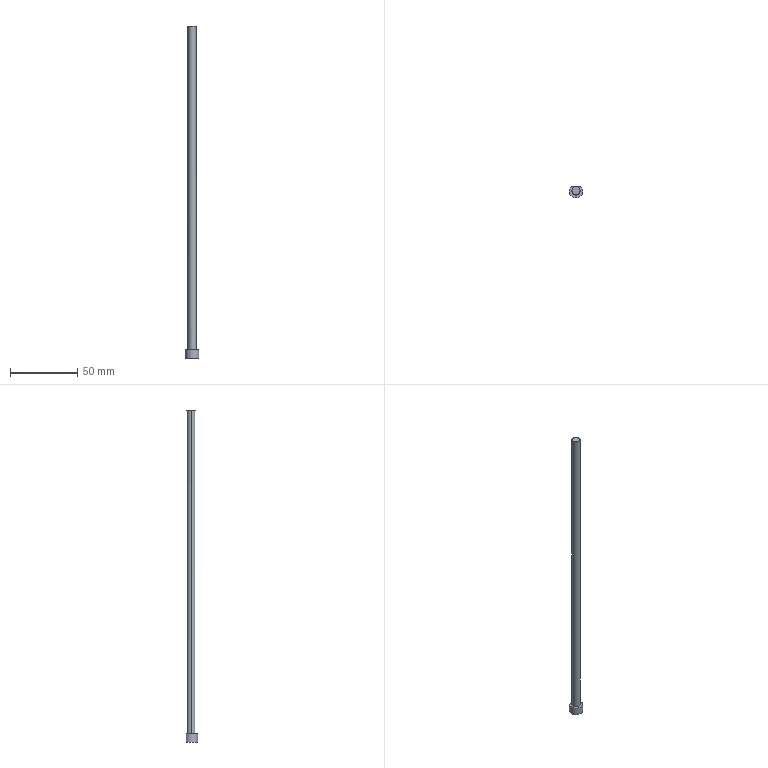Part | Creo | 1 solid | 7 faces | box 10 x 8.5 x 247.026 mm | volume 7242 mm3 | plane 4 | cylinder 3 | commonest cylinder face diameters 6 x2 10 x1
STEP:
#1=CARTESIAN_POINT('',(0.,0.,0.));
#2=DIRECTION('',(0.,0.,1.));
#3=DIRECTION('',(1.,0.,0.));
#4=AXIS2_PLACEMENT_3D('',#1,#2,#3);
#5=CARTESIAN_POINT('',(-69.606,-19.357,-332.441));
#6=VERTEX_POINT('',#5);
#7=CARTESIAN_POINT('',(-76.747,-19.357,-332.441));
#8=VERTEX_POINT('',#7);
#9=CARTESIAN_POINT('',(-69.606,-19.357,-332.441));
#10=DIRECTION('',(-1.,0.,0.));
#11=VECTOR('',#10,7.141);
#12=LINE('',#9,#11);
#13=EDGE_CURVE('',#6,#8,#12,.T.);
#14=ORIENTED_EDGE('',*,*,#13,.F.);
#15=CARTESIAN_POINT('',(-73.177,-22.857,-332.441));
#16=DIRECTION('',(0.,0.,-1.));
#17=DIRECTION('',(0.7141,0.7,0.));
#18=AXIS2_PLACEMENT_3D('',#15,#16,#17);
#19=CIRCLE('',#18,5.);
#20=EDGE_CURVE('',#6,#8,#19,.T.);
#21=ORIENTED_EDGE('',*,*,#20,.T.);
#22=EDGE_LOOP('',(#14,#21));
#23=FACE_OUTER_BOUND('',#22,.F.);
#24=CARTESIAN_POINT('',(-76.177,-22.857,-332.441));
#25=VERTEX_POINT('',#24);
#26=CARTESIAN_POINT('',(-70.177,-22.857,-332.441));
#27=VERTEX_POINT('',#26);
#28=CARTESIAN_POINT('',(-73.177,-22.857,-332.441));
#29=DIRECTION('',(0.,0.,-1.));
#30=DIRECTION('',(-1.,0.,0.));
#31=AXIS2_PLACEMENT_3D('',#28,#29,#30);
#32=CIRCLE('',#31,3.);
#33=EDGE_CURVE('',#25,#27,#32,.T.);
#34=ORIENTED_EDGE('',*,*,#33,.F.);
#35=CARTESIAN_POINT('',(-73.177,-22.857,-332.441));
#36=DIRECTION('',(0.,0.,-1.));
#37=DIRECTION('',(1.,0.,0.));
#38=AXIS2_PLACEMENT_3D('',#35,#36,#37);
#39=CIRCLE('',#38,3.);
#40=EDGE_CURVE('',#27,#25,#39,.T.);
#41=ORIENTED_EDGE('',*,*,#40,.F.);
#42=EDGE_LOOP('',(#34,#41));
#43=FACE_BOUND('',#42,.F.);
#44=CARTESIAN_POINT('',(-73.177,-22.857,-332.441));
#45=DIRECTION('',(0.,0.,-1.));
#46=DIRECTION('',(-1.,0.,0.));
#47=AXIS2_PLACEMENT_3D('',#44,#45,#46);
#48=PLANE('',#47);
#49=ADVANCED_FACE('',(#23,#43),#48,.F.);
#50=CARTESIAN_POINT('',(-70.177,-22.857,-91.423));
#51=VERTEX_POINT('',#50);
#52=CARTESIAN_POINT('',(-76.177,-22.856,-91.415));
#53=VERTEX_POINT('',#52);
#54=CARTESIAN_POINT('',(-70.177,-22.857,-91.423));
#55=CARTESIAN_POINT('',(-70.177,-22.528,-91.423));
#56=CARTESIAN_POINT('',(-70.279,-21.908,-91.423));
#57=CARTESIAN_POINT('',(-70.718,-21.051,-91.422));
#58=CARTESIAN_POINT('',(-71.395,-20.383,-91.421));
#59=CARTESIAN_POINT('',(-72.241,-19.955,-91.42));
#60=CARTESIAN_POINT('',(-73.175,-19.808,-91.419));
#61=CARTESIAN_POINT('',(-74.109,-19.954,-91.418));
#62=CARTESIAN_POINT('',(-74.956,-20.381,-91.417));
#63=CARTESIAN_POINT('',(-75.633,-21.048,-91.416));
#64=CARTESIAN_POINT('',(-76.073,-21.903,-91.415));
#65=CARTESIAN_POINT('',(-76.177,-22.527,-91.415));
#66=CARTESIAN_POINT('',(-76.177,-22.856,-91.415));
#67=B_SPLINE_CURVE_WITH_KNOTS('',3,(#54,#55,#56,#57,#58,#59,#60,#61,#62,#63,#64,#65,#66),.UNSPECIFIED.,.F.,.F.,(4,1,1,1,1,1,1,1,1,1,4),(0.,0.1,0.2,0.3,0.4,0.5,0.6,0.7,0.8,0.9,1.),.UNSPECIFIED.);
#68=EDGE_CURVE('',#51,#53,#67,.T.);
#69=ORIENTED_EDGE('',*,*,#68,.T.);
#70=CARTESIAN_POINT('',(-76.177,-22.857,-332.441));
#71=DIRECTION('',(0.000000003,0.000005265,1.));
#72=VECTOR('',#71,241.026);
#73=LINE('',#70,#72);
#74=EDGE_CURVE('',#25,#53,#73,.T.);
#75=ORIENTED_EDGE('',*,*,#74,.F.);
#76=ORIENTED_EDGE('',*,*,#33,.T.);
#77=CARTESIAN_POINT('',(-70.177,-22.857,-332.441));
#78=DIRECTION('',(0.,0.,1.));
#79=VECTOR('',#78,241.019);
#80=LINE('',#77,#79);
#81=EDGE_CURVE('',#27,#51,#80,.T.);
#82=ORIENTED_EDGE('',*,*,#81,.T.);
#83=EDGE_LOOP('',(#69,#75,#76,#82));
#84=FACE_OUTER_BOUND('',#83,.F.);
#85=CARTESIAN_POINT('',(-73.177,-22.857,-653.441));
#86=DIRECTION('',(0.,0.,1.));
#87=DIRECTION('',(1.,0.,0.));
#88=AXIS2_PLACEMENT_3D('',#85,#86,#87);
#89=CYLINDRICAL_SURFACE('',#88,3.);
#90=ADVANCED_FACE('',(#84),#89,.T.);
#91=CARTESIAN_POINT('',(-76.177,-22.856,-91.415));
#92=CARTESIAN_POINT('',(-76.177,-23.186,-91.415));
#93=CARTESIAN_POINT('',(-76.075,-23.804,-91.415));
#94=CARTESIAN_POINT('',(-75.636,-24.661,-91.416));
#95=CARTESIAN_POINT('',(-74.97,-25.322,-91.417));
#96=CARTESIAN_POINT('',(-74.131,-25.754,-91.418));
#97=CARTESIAN_POINT('',(-73.189,-25.907,-91.419));
#98=CARTESIAN_POINT('',(-72.247,-25.761,-91.42));
#99=CARTESIAN_POINT('',(-71.402,-25.336,-91.421));
#100=CARTESIAN_POINT('',(-70.725,-24.674,-91.422));
#101=CARTESIAN_POINT('',(-70.279,-23.807,-91.423));
#102=CARTESIAN_POINT('',(-70.177,-23.186,-91.423));
#103=CARTESIAN_POINT('',(-70.177,-22.857,-91.423));
#104=B_SPLINE_CURVE_WITH_KNOTS('',3,(#91,#92,#93,#94,#95,#96,#97,#98,#99,#100,#101,#102,#103),.UNSPECIFIED.,.F.,.F.,(4,1,1,1,1,1,1,1,1,1,4),(0.,0.1,0.2,0.3,0.4,0.5,0.6,0.7,0.8,0.9,1.),.UNSPECIFIED.);
#105=EDGE_CURVE('',#53,#51,#104,.T.);
#106=ORIENTED_EDGE('',*,*,#105,.F.);
#107=ORIENTED_EDGE('',*,*,#68,.F.);
#108=EDGE_LOOP('',(#106,#107));
#109=FACE_OUTER_BOUND('',#108,.F.);
#110=CARTESIAN_POINT('',(248.993,54.022,-91.842));
#111=DIRECTION('',(-0.001312,0.000001665,-1.));
#112=DIRECTION('',(-1.,0.,0.001312));
#113=AXIS2_PLACEMENT_3D('',#110,#111,#112);
#114=PLANE('',#113);
#115=ADVANCED_FACE('',(#109),#114,.F.);
#116=ORIENTED_EDGE('',*,*,#105,.T.);
#117=ORIENTED_EDGE('',*,*,#81,.F.);
#118=ORIENTED_EDGE('',*,*,#40,.T.);
#119=ORIENTED_EDGE('',*,*,#74,.T.);
#120=EDGE_LOOP('',(#116,#117,#118,#119));
#121=FACE_OUTER_BOUND('',#120,.F.);
#122=CARTESIAN_POINT('',(-73.177,-22.857,-653.441));
#123=DIRECTION('',(0.,0.,1.));
#124=DIRECTION('',(1.,0.,0.));
#125=AXIS2_PLACEMENT_3D('',#122,#123,#124);
#126=CYLINDRICAL_SURFACE('',#125,3.);
#127=ADVANCED_FACE('',(#121),#126,.T.);
#128=CARTESIAN_POINT('',(-76.747,-19.357,-338.441));
#129=VERTEX_POINT('',#128);
#130=CARTESIAN_POINT('',(-76.747,-19.357,-332.441));
#131=DIRECTION('',(0.,0.,-1.));
#132=VECTOR('',#131,6.);
#133=LINE('',#130,#132);
#134=EDGE_CURVE('',#8,#129,#133,.T.);
#135=ORIENTED_EDGE('',*,*,#134,.T.);
#136=CARTESIAN_POINT('',(-69.606,-19.357,-338.441));
#137=VERTEX_POINT('',#136);
#138=CARTESIAN_POINT('',(-69.606,-19.357,-338.441));
#139=DIRECTION('',(-1.,0.,0.));
#140=VECTOR('',#139,7.141);
#141=LINE('',#138,#140);
#142=EDGE_CURVE('',#137,#129,#141,.T.);
#143=ORIENTED_EDGE('',*,*,#142,.F.);
#144=CARTESIAN_POINT('',(-69.606,-19.357,-338.441));
#145=DIRECTION('',(0.,0.,1.));
#146=VECTOR('',#145,6.);
#147=LINE('',#144,#146);
#148=EDGE_CURVE('',#137,#6,#147,.T.);
#149=ORIENTED_EDGE('',*,*,#148,.T.);
#150=ORIENTED_EDGE('',*,*,#13,.T.);
#151=EDGE_LOOP('',(#135,#143,#149,#150));
#152=FACE_OUTER_BOUND('',#151,.F.);
#153=CARTESIAN_POINT('',(-73.177,-19.357,-338.441));
#154=DIRECTION('',(0.,1.,0.));
#155=DIRECTION('',(0.,0.,1.));
#156=AXIS2_PLACEMENT_3D('',#153,#154,#155);
#157=PLANE('',#156);
#158=ADVANCED_FACE('',(#152),#157,.T.);
#159=CARTESIAN_POINT('',(-73.177,-22.857,-338.441));
#160=DIRECTION('',(0.,0.,1.));
#161=DIRECTION('',(-0.7141,0.7,0.));
#162=AXIS2_PLACEMENT_3D('',#159,#160,#161);
#163=CIRCLE('',#162,5.);
#164=EDGE_CURVE('',#129,#137,#163,.T.);
#165=ORIENTED_EDGE('',*,*,#164,.F.);
#166=ORIENTED_EDGE('',*,*,#134,.F.);
#167=ORIENTED_EDGE('',*,*,#20,.F.);
#168=ORIENTED_EDGE('',*,*,#148,.F.);
#169=EDGE_LOOP('',(#165,#166,#167,#168));
#170=FACE_OUTER_BOUND('',#169,.F.);
#171=CARTESIAN_POINT('',(-73.177,-22.857,-332.441));
#172=DIRECTION('',(0.,0.,-1.));
#173=DIRECTION('',(-1.,0.,0.));
#174=AXIS2_PLACEMENT_3D('',#171,#172,#173);
#175=CYLINDRICAL_SURFACE('',#174,5.);
#176=ADVANCED_FACE('',(#170),#175,.T.);
#177=ORIENTED_EDGE('',*,*,#164,.T.);
#178=ORIENTED_EDGE('',*,*,#142,.T.);
#179=EDGE_LOOP('',(#177,#178));
#180=FACE_OUTER_BOUND('',#179,.F.);
#181=CARTESIAN_POINT('',(-73.177,-22.857,-338.441));
#182=DIRECTION('',(0.,0.,-1.));
#183=DIRECTION('',(-1.,0.,0.));
#184=AXIS2_PLACEMENT_3D('',#181,#182,#183);
#185=PLANE('',#184);
#186=ADVANCED_FACE('',(#180),#185,.T.);
#187=CLOSED_SHELL('',(#49,#90,#115,#127,#158,#176,#186));
#188=MANIFOLD_SOLID_BREP('',#187);
#189=(LENGTH_UNIT()NAMED_UNIT(*)SI_UNIT(.MILLI.,.METRE.));
#190=UNCERTAINTY_MEASURE_WITH_UNIT(LENGTH_MEASURE(0.02474),#189,'','');
#191=(NAMED_UNIT(*)PLANE_ANGLE_UNIT()SI_UNIT($,.RADIAN.));
#192=PLANE_ANGLE_MEASURE_WITH_UNIT(PLANE_ANGLE_MEASURE(0.01745),#191);
#193=(CONVERSION_BASED_UNIT('DEGREE',#192)NAMED_UNIT(*)PLANE_ANGLE_UNIT());
#194=(NAMED_UNIT(*)SI_UNIT($,.STERADIAN.)SOLID_ANGLE_UNIT());
#195=(GEOMETRIC_REPRESENTATION_CONTEXT(3)GLOBAL_UNCERTAINTY_ASSIGNED_CONTEXT((#190))GLOBAL_UNIT_ASSIGNED_CONTEXT((#189,#193,#194))REPRESENTATION_CONTEXT('',''));
#196=ADVANCED_BREP_SHAPE_REPRESENTATION('',(#4,#188),#195);